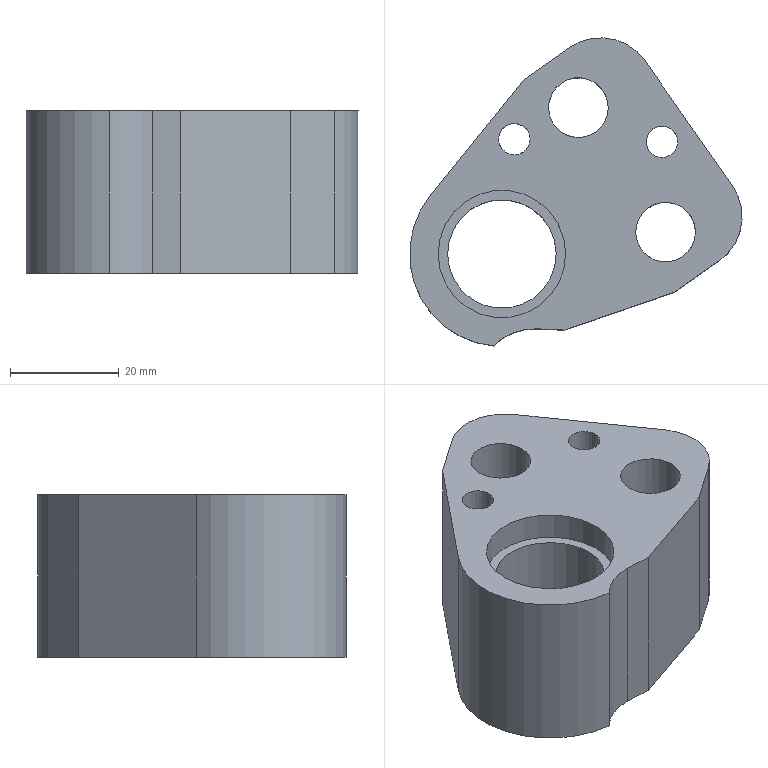Part | NX | features solid 2 | 1 solid | 27 faces | box 61.243 x 56.752 x 30 mm | volume 46658 mm3 | cylinder 14 | plane 13 | commonest cylinder face diameters 20 x3 5.8 x2 8 x2 11 x2 17 x2 21 x1
STEP:
#1=CARTESIAN_POINT('',(-510.031,-151.839,44.));
#2=VERTEX_POINT('',#1);
#3=CARTESIAN_POINT('',(-510.031,-151.839,74.));
#4=VERTEX_POINT('',#3);
#5=CARTESIAN_POINT('',(-510.031,-151.839,44.));
#6=DIRECTION('',(0.,0.,1.));
#7=VECTOR('',#6,1000.);
#8=LINE('',#5,#7);
#9=EDGE_CURVE('',#2,#4,#8,.T.);
#10=ORIENTED_EDGE('',*,*,#9,.F.);
#11=CARTESIAN_POINT('',(-489.755,-144.863,44.));
#12=VERTEX_POINT('',#11);
#13=CARTESIAN_POINT('',(-508.667,-151.37,44.));
#14=DIRECTION('',(-0.9456,-0.3254,0.));
#15=VECTOR('',#14,1000.);
#16=LINE('',#13,#15);
#17=EDGE_CURVE('',#12,#2,#16,.T.);
#18=ORIENTED_EDGE('',*,*,#17,.F.);
#19=CARTESIAN_POINT('',(-489.755,-144.863,74.));
#20=VERTEX_POINT('',#19);
#21=CARTESIAN_POINT('',(-489.755,-144.863,44.));
#22=DIRECTION('',(0.,0.,1.));
#23=VECTOR('',#22,1000.);
#24=LINE('',#21,#23);
#25=EDGE_CURVE('',#12,#20,#24,.T.);
#26=ORIENTED_EDGE('',*,*,#25,.T.);
#27=CARTESIAN_POINT('',(-508.667,-151.37,74.));
#28=DIRECTION('',(0.9456,0.3254,0.));
#29=VECTOR('',#28,1000.);
#30=LINE('',#27,#29);
#31=EDGE_CURVE('',#4,#20,#30,.T.);
#32=ORIENTED_EDGE('',*,*,#31,.F.);
#33=EDGE_LOOP('',(#10,#18,#26,#32));
#34=FACE_BOUND('',#33,.T.);
#35=CARTESIAN_POINT('',(-508.667,-151.37,44.));
#36=DIRECTION('',(-0.3254,0.9456,0.));
#37=DIRECTION('',(0.,0.,-1.));
#38=AXIS2_PLACEMENT_3D('',#35,#36,#37);
#39=PLANE('',#38);
#40=ADVANCED_FACE('',(#34),#39,.F.);
#41=CARTESIAN_POINT('',(-515.152,-151.612,74.));
#42=VERTEX_POINT('',#41);
#43=CARTESIAN_POINT('',(-523.093,-154.751,74.));
#44=VERTEX_POINT('',#43);
#45=CARTESIAN_POINT('',(-515.596,-162.103,74.));
#46=DIRECTION('',(0.,0.,1.));
#47=DIRECTION('',(0.,-1.,0.));
#48=AXIS2_PLACEMENT_3D('',#45,#46,#47);
#49=CIRCLE('',#48,10.5);
#50=EDGE_CURVE('',#42,#44,#49,.T.);
#51=ORIENTED_EDGE('',*,*,#50,.F.);
#52=CARTESIAN_POINT('',(-515.285,-151.606,74.));
#53=DIRECTION('',(0.999,-0.04437,0.));
#54=VECTOR('',#53,1000.);
#55=LINE('',#52,#54);
#56=EDGE_CURVE('',#42,#4,#55,.T.);
#57=ORIENTED_EDGE('',*,*,#56,.T.);
#58=ORIENTED_EDGE('',*,*,#31,.T.);
#59=CARTESIAN_POINT('',(-481.564,-139.127,74.));
#60=VERTEX_POINT('',#59);
#61=CARTESIAN_POINT('',(-500.687,-152.517,74.));
#62=DIRECTION('',(-0.8192,-0.5736,0.));
#63=VECTOR('',#62,1000.);
#64=LINE('',#61,#63);
#65=EDGE_CURVE('',#60,#20,#64,.T.);
#66=ORIENTED_EDGE('',*,*,#65,.F.);
#67=CARTESIAN_POINT('',(-479.108,-125.2,74.));
#68=VERTEX_POINT('',#67);
#69=CARTESIAN_POINT('',(-487.299,-130.936,74.));
#70=DIRECTION('',(0.,0.,1.));
#71=DIRECTION('',(0.,-1.,0.));
#72=AXIS2_PLACEMENT_3D('',#69,#70,#71);
#73=CIRCLE('',#72,10.);
#74=EDGE_CURVE('',#60,#68,#73,.T.);
#75=ORIENTED_EDGE('',*,*,#74,.T.);
#76=CARTESIAN_POINT('',(-495.168,-102.264,74.));
#77=VERTEX_POINT('',#76);
#78=CARTESIAN_POINT('',(-487.138,-113.732,74.));
#79=DIRECTION('',(0.5736,-0.8192,0.));
#80=VECTOR('',#79,1000.);
#81=LINE('',#78,#80);
#82=EDGE_CURVE('',#77,#68,#81,.T.);
#83=ORIENTED_EDGE('',*,*,#82,.F.);
#84=CARTESIAN_POINT('',(-509.095,-99.808,74.));
#85=VERTEX_POINT('',#84);
#86=CARTESIAN_POINT('',(-503.359,-107.999,74.));
#87=DIRECTION('',(0.,0.,1.));
#88=DIRECTION('',(0.,-1.,0.));
#89=AXIS2_PLACEMENT_3D('',#86,#87,#88);
#90=CIRCLE('',#89,10.);
#91=EDGE_CURVE('',#77,#85,#90,.T.);
#92=ORIENTED_EDGE('',*,*,#91,.T.);
#93=CARTESIAN_POINT('',(-517.287,-105.544,74.));
#94=VERTEX_POINT('',#93);
#95=CARTESIAN_POINT('',(-528.218,-113.198,74.));
#96=DIRECTION('',(0.8192,0.5736,0.));
#97=VECTOR('',#96,1000.);
#98=LINE('',#95,#97);
#99=EDGE_CURVE('',#94,#85,#98,.T.);
#100=ORIENTED_EDGE('',*,*,#99,.F.);
#101=CARTESIAN_POINT('',(-534.756,-127.127,74.));
#102=VERTEX_POINT('',#101);
#103=CARTESIAN_POINT('',(-529.87,-121.089,74.));
#104=DIRECTION('',(-0.6291,-0.7773,0.));
#105=VECTOR('',#104,1000.);
#106=LINE('',#103,#105);
#107=EDGE_CURVE('',#94,#102,#106,.T.);
#108=ORIENTED_EDGE('',*,*,#107,.T.);
#109=CARTESIAN_POINT('',(-521.542,-137.822,74.));
#110=DIRECTION('',(0.,0.,-1.));
#111=DIRECTION('',(0.5736,-0.8192,0.));
#112=AXIS2_PLACEMENT_3D('',#109,#110,#111);
#113=CIRCLE('',#112,17.);
#114=EDGE_CURVE('',#44,#102,#113,.T.);
#115=ORIENTED_EDGE('',*,*,#114,.F.);
#116=EDGE_LOOP('',(#51,#57,#58,#66,#75,#83,#92,#100,#108,#115));
#117=FACE_BOUND('',#116,.T.);
#118=CARTESIAN_POINT('',(-490.389,-119.549,74.));
#119=VERTEX_POINT('',#118);
#120=CARTESIAN_POINT('',(-492.053,-117.173,74.));
#121=DIRECTION('',(0.,0.,-1.));
#122=DIRECTION('',(0.5736,-0.8192,0.));
#123=AXIS2_PLACEMENT_3D('',#120,#121,#122);
#124=CIRCLE('',#123,2.9);
#125=EDGE_CURVE('',#119,#119,#124,.T.);
#126=ORIENTED_EDGE('',*,*,#125,.T.);
#127=EDGE_LOOP('',(#126));
#128=FACE_BOUND('',#127,.T.);
#129=CARTESIAN_POINT('',(-517.588,-119.061,74.));
#130=VERTEX_POINT('',#129);
#131=CARTESIAN_POINT('',(-519.251,-116.686,74.));
#132=DIRECTION('',(0.,0.,-1.));
#133=DIRECTION('',(0.5736,-0.8192,0.));
#134=AXIS2_PLACEMENT_3D('',#131,#132,#133);
#135=CIRCLE('',#134,2.9);
#136=EDGE_CURVE('',#130,#130,#135,.T.);
#137=ORIENTED_EDGE('',*,*,#136,.T.);
#138=EDGE_LOOP('',(#137));
#139=FACE_BOUND('',#138,.T.);
#140=CARTESIAN_POINT('',(-504.301,-115.373,74.));
#141=VERTEX_POINT('',#140);
#142=CARTESIAN_POINT('',(-507.455,-110.867,74.));
#143=DIRECTION('',(0.,0.,-1.));
#144=DIRECTION('',(0.5736,-0.8192,0.));
#145=AXIS2_PLACEMENT_3D('',#142,#143,#144);
#146=CIRCLE('',#145,5.5);
#147=EDGE_CURVE('',#141,#141,#146,.T.);
#148=ORIENTED_EDGE('',*,*,#147,.T.);
#149=EDGE_LOOP('',(#148));
#150=FACE_BOUND('',#149,.T.);
#151=CARTESIAN_POINT('',(-488.24,-138.309,74.));
#152=VERTEX_POINT('',#151);
#153=CARTESIAN_POINT('',(-491.395,-133.804,74.));
#154=DIRECTION('',(0.,0.,-1.));
#155=DIRECTION('',(0.5736,-0.8192,0.));
#156=AXIS2_PLACEMENT_3D('',#153,#154,#155);
#157=CIRCLE('',#156,5.5);
#158=EDGE_CURVE('',#152,#152,#157,.T.);
#159=ORIENTED_EDGE('',*,*,#158,.T.);
#160=EDGE_LOOP('',(#159));
#161=FACE_BOUND('',#160,.T.);
#162=CARTESIAN_POINT('',(-514.803,-147.447,74.));
#163=VERTEX_POINT('',#162);
#164=CARTESIAN_POINT('',(-521.542,-137.822,74.));
#165=DIRECTION('',(0.,0.,-1.));
#166=DIRECTION('',(0.5736,-0.8192,0.));
#167=AXIS2_PLACEMENT_3D('',#164,#165,#166);
#168=CIRCLE('',#167,11.75);
#169=EDGE_CURVE('',#163,#163,#168,.T.);
#170=ORIENTED_EDGE('',*,*,#169,.T.);
#171=EDGE_LOOP('',(#170));
#172=FACE_BOUND('',#171,.T.);
#173=CARTESIAN_POINT('',(-514.453,-132.858,74.));
#174=DIRECTION('',(0.,0.,1.));
#175=DIRECTION('',(-0.5736,0.8192,0.));
#176=AXIS2_PLACEMENT_3D('',#173,#174,#175);
#177=PLANE('',#176);
#178=ADVANCED_FACE('',(#117,#128,#139,#150,#161,#172),#177,.T.);
#179=ORIENTED_EDGE('',*,*,#25,.F.);
#180=CARTESIAN_POINT('',(-481.564,-139.127,44.));
#181=VERTEX_POINT('',#180);
#182=CARTESIAN_POINT('',(-500.687,-152.517,44.));
#183=DIRECTION('',(0.8192,0.5736,0.));
#184=VECTOR('',#183,1000.);
#185=LINE('',#182,#184);
#186=EDGE_CURVE('',#12,#181,#185,.T.);
#187=ORIENTED_EDGE('',*,*,#186,.T.);
#188=CARTESIAN_POINT('',(-481.564,-139.127,44.));
#189=DIRECTION('',(0.,0.,1.));
#190=VECTOR('',#189,1000.);
#191=LINE('',#188,#190);
#192=EDGE_CURVE('',#181,#60,#191,.T.);
#193=ORIENTED_EDGE('',*,*,#192,.T.);
#194=ORIENTED_EDGE('',*,*,#65,.T.);
#195=EDGE_LOOP('',(#179,#187,#193,#194));
#196=FACE_BOUND('',#195,.T.);
#197=CARTESIAN_POINT('',(-500.687,-152.517,44.));
#198=DIRECTION('',(0.5736,-0.8192,0.));
#199=DIRECTION('',(0.,0.,1.));
#200=AXIS2_PLACEMENT_3D('',#197,#198,#199);
#201=PLANE('',#200);
#202=ADVANCED_FACE('',(#196),#201,.T.);
#203=CARTESIAN_POINT('',(-523.093,-154.751,44.));
#204=VERTEX_POINT('',#203);
#205=CARTESIAN_POINT('',(-515.152,-151.612,44.));
#206=VERTEX_POINT('',#205);
#207=CARTESIAN_POINT('',(-515.596,-162.103,44.));
#208=DIRECTION('',(0.,0.,-1.));
#209=DIRECTION('',(0.,1.,0.));
#210=AXIS2_PLACEMENT_3D('',#207,#208,#209);
#211=CIRCLE('',#210,10.5);
#212=EDGE_CURVE('',#204,#206,#211,.T.);
#213=ORIENTED_EDGE('',*,*,#212,.F.);
#214=CARTESIAN_POINT('',(-534.756,-127.127,44.));
#215=VERTEX_POINT('',#214);
#216=CARTESIAN_POINT('',(-521.542,-137.822,44.));
#217=DIRECTION('',(0.,0.,1.));
#218=DIRECTION('',(-0.5736,0.8192,0.));
#219=AXIS2_PLACEMENT_3D('',#216,#217,#218);
#220=CIRCLE('',#219,17.);
#221=EDGE_CURVE('',#215,#204,#220,.T.);
#222=ORIENTED_EDGE('',*,*,#221,.F.);
#223=CARTESIAN_POINT('',(-517.287,-105.544,44.));
#224=VERTEX_POINT('',#223);
#225=CARTESIAN_POINT('',(-529.87,-121.089,44.));
#226=DIRECTION('',(0.6291,0.7773,0.));
#227=VECTOR('',#226,1000.);
#228=LINE('',#225,#227);
#229=EDGE_CURVE('',#215,#224,#228,.T.);
#230=ORIENTED_EDGE('',*,*,#229,.T.);
#231=CARTESIAN_POINT('',(-509.095,-99.808,44.));
#232=VERTEX_POINT('',#231);
#233=CARTESIAN_POINT('',(-528.218,-113.198,44.));
#234=DIRECTION('',(-0.8192,-0.5736,0.));
#235=VECTOR('',#234,1000.);
#236=LINE('',#233,#235);
#237=EDGE_CURVE('',#232,#224,#236,.T.);
#238=ORIENTED_EDGE('',*,*,#237,.F.);
#239=CARTESIAN_POINT('',(-495.168,-102.264,44.));
#240=VERTEX_POINT('',#239);
#241=CARTESIAN_POINT('',(-503.359,-107.999,44.));
#242=DIRECTION('',(0.,0.,-1.));
#243=DIRECTION('',(0.,1.,0.));
#244=AXIS2_PLACEMENT_3D('',#241,#242,#243);
#245=CIRCLE('',#244,10.);
#246=EDGE_CURVE('',#232,#240,#245,.T.);
#247=ORIENTED_EDGE('',*,*,#246,.T.);
#248=CARTESIAN_POINT('',(-479.108,-125.2,44.));
#249=VERTEX_POINT('',#248);
#250=CARTESIAN_POINT('',(-487.138,-113.732,44.));
#251=DIRECTION('',(-0.5736,0.8192,0.));
#252=VECTOR('',#251,1000.);
#253=LINE('',#250,#252);
#254=EDGE_CURVE('',#249,#240,#253,.T.);
#255=ORIENTED_EDGE('',*,*,#254,.F.);
#256=CARTESIAN_POINT('',(-487.299,-130.936,44.));
#257=DIRECTION('',(0.,0.,-1.));
#258=DIRECTION('',(0.,1.,0.));
#259=AXIS2_PLACEMENT_3D('',#256,#257,#258);
#260=CIRCLE('',#259,10.);
#261=EDGE_CURVE('',#249,#181,#260,.T.);
#262=ORIENTED_EDGE('',*,*,#261,.T.);
#263=ORIENTED_EDGE('',*,*,#186,.F.);
#264=ORIENTED_EDGE('',*,*,#17,.T.);
#265=CARTESIAN_POINT('',(-515.285,-151.606,44.));
#266=DIRECTION('',(-0.999,0.04437,0.));
#267=VECTOR('',#266,1000.);
#268=LINE('',#265,#267);
#269=EDGE_CURVE('',#2,#206,#268,.T.);
#270=ORIENTED_EDGE('',*,*,#269,.T.);
#271=EDGE_LOOP('',(#213,#222,#230,#238,#247,#255,#262,#263,#264,#270));
#272=FACE_BOUND('',#271,.T.);
#273=CARTESIAN_POINT('',(-494.347,-113.897,44.));
#274=VERTEX_POINT('',#273);
#275=CARTESIAN_POINT('',(-492.053,-117.173,44.));
#276=DIRECTION('',(0.,0.,1.));
#277=DIRECTION('',(-0.5736,0.8192,0.));
#278=AXIS2_PLACEMENT_3D('',#275,#276,#277);
#279=CIRCLE('',#278,4.);
#280=EDGE_CURVE('',#274,#274,#279,.T.);
#281=ORIENTED_EDGE('',*,*,#280,.T.);
#282=EDGE_LOOP('',(#281));
#283=FACE_BOUND('',#282,.T.);
#284=CARTESIAN_POINT('',(-521.546,-113.409,44.));
#285=VERTEX_POINT('',#284);
#286=CARTESIAN_POINT('',(-519.251,-116.686,44.));
#287=DIRECTION('',(0.,0.,1.));
#288=DIRECTION('',(-0.5736,0.8192,0.));
#289=AXIS2_PLACEMENT_3D('',#286,#287,#288);
#290=CIRCLE('',#289,4.);
#291=EDGE_CURVE('',#285,#285,#290,.T.);
#292=ORIENTED_EDGE('',*,*,#291,.T.);
#293=EDGE_LOOP('',(#292));
#294=FACE_BOUND('',#293,.T.);
#295=CARTESIAN_POINT('',(-512.331,-103.905,44.));
#296=VERTEX_POINT('',#295);
#297=CARTESIAN_POINT('',(-507.455,-110.867,44.));
#298=DIRECTION('',(0.,0.,1.));
#299=DIRECTION('',(-0.5736,0.8192,0.));
#300=AXIS2_PLACEMENT_3D('',#297,#298,#299);
#301=CIRCLE('',#300,8.5);
#302=EDGE_CURVE('',#296,#296,#301,.T.);
#303=ORIENTED_EDGE('',*,*,#302,.T.);
#304=EDGE_LOOP('',(#303));
#305=FACE_BOUND('',#304,.T.);
#306=CARTESIAN_POINT('',(-496.271,-126.841,44.));
#307=VERTEX_POINT('',#306);
#308=CARTESIAN_POINT('',(-491.395,-133.804,44.));
#309=DIRECTION('',(0.,0.,1.));
#310=DIRECTION('',(-0.5736,0.8192,0.));
#311=AXIS2_PLACEMENT_3D('',#308,#309,#310);
#312=CIRCLE('',#311,8.5);
#313=EDGE_CURVE('',#307,#307,#312,.T.);
#314=ORIENTED_EDGE('',*,*,#313,.T.);
#315=EDGE_LOOP('',(#314));
#316=FACE_BOUND('',#315,.T.);
#317=CARTESIAN_POINT('',(-527.278,-129.631,44.));
#318=VERTEX_POINT('',#317);
#319=CARTESIAN_POINT('',(-521.542,-137.822,44.));
#320=DIRECTION('',(0.,0.,1.));
#321=DIRECTION('',(-0.5736,0.8192,0.));
#322=AXIS2_PLACEMENT_3D('',#319,#320,#321);
#323=CIRCLE('',#322,10.);
#324=EDGE_CURVE('',#318,#318,#323,.T.);
#325=ORIENTED_EDGE('',*,*,#324,.T.);
#326=EDGE_LOOP('',(#325));
#327=FACE_BOUND('',#326,.T.);
#328=CARTESIAN_POINT('',(-514.453,-132.858,44.));
#329=DIRECTION('',(0.,0.,-1.));
#330=DIRECTION('',(0.5736,-0.8192,0.));
#331=AXIS2_PLACEMENT_3D('',#328,#329,#330);
#332=PLANE('',#331);
#333=ADVANCED_FACE('',(#272,#283,#294,#305,#316,#327),#332,.T.);
#334=CARTESIAN_POINT('',(-517.287,-105.544,44.));
#335=DIRECTION('',(0.,0.,1.));
#336=VECTOR('',#335,1000.);
#337=LINE('',#334,#336);
#338=EDGE_CURVE('',#224,#94,#337,.T.);
#339=ORIENTED_EDGE('',*,*,#338,.T.);
#340=ORIENTED_EDGE('',*,*,#99,.T.);
#341=CARTESIAN_POINT('',(-509.095,-99.808,44.));
#342=DIRECTION('',(0.,0.,1.));
#343=VECTOR('',#342,1000.);
#344=LINE('',#341,#343);
#345=EDGE_CURVE('',#85,#232,#344,.F.);
#346=ORIENTED_EDGE('',*,*,#345,.T.);
#347=ORIENTED_EDGE('',*,*,#237,.T.);
#348=EDGE_LOOP('',(#339,#340,#346,#347));
#349=FACE_BOUND('',#348,.T.);
#350=CARTESIAN_POINT('',(-528.218,-113.198,44.));
#351=DIRECTION('',(-0.5736,0.8192,0.));
#352=DIRECTION('',(0.,0.,-1.));
#353=AXIS2_PLACEMENT_3D('',#350,#351,#352);
#354=PLANE('',#353);
#355=ADVANCED_FACE('',(#349),#354,.T.);
#356=CARTESIAN_POINT('',(-523.093,-154.751,150.));
#357=DIRECTION('',(0.,0.,1.));
#358=VECTOR('',#357,1000.);
#359=LINE('',#356,#358);
#360=EDGE_CURVE('',#44,#204,#359,.F.);
#361=ORIENTED_EDGE('',*,*,#360,.F.);
#362=ORIENTED_EDGE('',*,*,#114,.T.);
#363=CARTESIAN_POINT('',(-534.756,-127.127,74.));
#364=DIRECTION('',(0.,0.,-1.));
#365=VECTOR('',#364,1000.);
#366=LINE('',#363,#365);
#367=EDGE_CURVE('',#102,#215,#366,.T.);
#368=ORIENTED_EDGE('',*,*,#367,.T.);
#369=ORIENTED_EDGE('',*,*,#221,.T.);
#370=EDGE_LOOP('',(#361,#362,#368,#369));
#371=FACE_BOUND('',#370,.T.);
#372=CARTESIAN_POINT('',(-521.542,-137.822,74.));
#373=DIRECTION('',(0.,0.,-1.));
#374=DIRECTION('',(0.5736,-0.8192,0.));
#375=AXIS2_PLACEMENT_3D('',#372,#373,#374);
#376=CYLINDRICAL_SURFACE('',#375,17.);
#377=ADVANCED_FACE('',(#371),#376,.T.);
#378=ORIENTED_EDGE('',*,*,#254,.T.);
#379=CARTESIAN_POINT('',(-495.168,-102.264,44.));
#380=DIRECTION('',(0.,0.,1.));
#381=VECTOR('',#380,1000.);
#382=LINE('',#379,#381);
#383=EDGE_CURVE('',#240,#77,#382,.T.);
#384=ORIENTED_EDGE('',*,*,#383,.T.);
#385=ORIENTED_EDGE('',*,*,#82,.T.);
#386=CARTESIAN_POINT('',(-479.108,-125.2,44.));
#387=DIRECTION('',(0.,0.,1.));
#388=VECTOR('',#387,1000.);
#389=LINE('',#386,#388);
#390=EDGE_CURVE('',#68,#249,#389,.F.);
#391=ORIENTED_EDGE('',*,*,#390,.T.);
#392=EDGE_LOOP('',(#378,#384,#385,#391));
#393=FACE_BOUND('',#392,.T.);
#394=CARTESIAN_POINT('',(-487.138,-113.732,44.));
#395=DIRECTION('',(0.8192,0.5736,0.));
#396=DIRECTION('',(0.,0.,-1.));
#397=AXIS2_PLACEMENT_3D('',#394,#395,#396);
#398=PLANE('',#397);
#399=ADVANCED_FACE('',(#393),#398,.T.);
#400=CARTESIAN_POINT('',(-515.807,-146.014,69.));
#401=VERTEX_POINT('',#400);
#402=CARTESIAN_POINT('',(-521.542,-137.822,69.));
#403=DIRECTION('',(0.,0.,-1.));
#404=DIRECTION('',(0.5736,-0.8192,0.));
#405=AXIS2_PLACEMENT_3D('',#402,#403,#404);
#406=CIRCLE('',#405,10.);
#407=EDGE_CURVE('',#401,#401,#406,.T.);
#408=ORIENTED_EDGE('',*,*,#407,.T.);
#409=EDGE_LOOP('',(#408));
#410=FACE_BOUND('',#409,.T.);
#411=CARTESIAN_POINT('',(-528.282,-128.197,69.));
#412=VERTEX_POINT('',#411);
#413=CARTESIAN_POINT('',(-521.542,-137.822,69.));
#414=DIRECTION('',(0.,0.,1.));
#415=DIRECTION('',(-0.5736,0.8192,0.));
#416=AXIS2_PLACEMENT_3D('',#413,#414,#415);
#417=CIRCLE('',#416,11.75);
#418=EDGE_CURVE('',#412,#412,#417,.T.);
#419=ORIENTED_EDGE('',*,*,#418,.T.);
#420=EDGE_LOOP('',(#419));
#421=FACE_BOUND('',#420,.T.);
#422=CARTESIAN_POINT('',(-521.542,-137.822,69.));
#423=DIRECTION('',(0.,0.,-1.));
#424=DIRECTION('',(0.5736,-0.8192,0.));
#425=AXIS2_PLACEMENT_3D('',#422,#423,#424);
#426=PLANE('',#425);
#427=ADVANCED_FACE('',(#410,#421),#426,.F.);
#428=ORIENTED_EDGE('',*,*,#418,.F.);
#429=EDGE_LOOP('',(#428));
#430=FACE_BOUND('',#429,.T.);
#431=ORIENTED_EDGE('',*,*,#169,.F.);
#432=EDGE_LOOP('',(#431));
#433=FACE_BOUND('',#432,.T.);
#434=CARTESIAN_POINT('',(-521.542,-137.822,74.));
#435=DIRECTION('',(0.,0.,-1.));
#436=DIRECTION('',(0.5736,-0.8192,0.));
#437=AXIS2_PLACEMENT_3D('',#434,#435,#436);
#438=CYLINDRICAL_SURFACE('',#437,11.75);
#439=ADVANCED_FACE('',(#430,#433),#438,.F.);
#440=ORIENTED_EDGE('',*,*,#324,.F.);
#441=EDGE_LOOP('',(#440));
#442=FACE_BOUND('',#441,.T.);
#443=ORIENTED_EDGE('',*,*,#407,.F.);
#444=EDGE_LOOP('',(#443));
#445=FACE_BOUND('',#444,.T.);
#446=CARTESIAN_POINT('',(-521.542,-137.822,69.));
#447=DIRECTION('',(0.,0.,-1.));
#448=DIRECTION('',(0.5736,-0.8192,0.));
#449=AXIS2_PLACEMENT_3D('',#446,#447,#448);
#450=CYLINDRICAL_SURFACE('',#449,10.);
#451=ADVANCED_FACE('',(#442,#445),#450,.F.);
#452=CARTESIAN_POINT('',(-491.395,-139.304,56.));
#453=VERTEX_POINT('',#452);
#454=CARTESIAN_POINT('',(-491.395,-133.804,56.));
#455=DIRECTION('',(0.,0.,1.));
#456=DIRECTION('',(0.,-1.,0.));
#457=AXIS2_PLACEMENT_3D('',#454,#455,#456);
#458=CIRCLE('',#457,5.5);
#459=EDGE_CURVE('',#453,#453,#458,.F.);
#460=ORIENTED_EDGE('',*,*,#459,.T.);
#461=EDGE_LOOP('',(#460));
#462=FACE_BOUND('',#461,.T.);
#463=ORIENTED_EDGE('',*,*,#158,.F.);
#464=EDGE_LOOP('',(#463));
#465=FACE_BOUND('',#464,.T.);
#466=CARTESIAN_POINT('',(-491.395,-133.804,74.));
#467=DIRECTION('',(0.,0.,-1.));
#468=DIRECTION('',(0.5736,-0.8192,0.));
#469=AXIS2_PLACEMENT_3D('',#466,#467,#468);
#470=CYLINDRICAL_SURFACE('',#469,5.5);
#471=ADVANCED_FACE('',(#462,#465),#470,.F.);
#472=CARTESIAN_POINT('',(-486.52,-140.766,56.));
#473=VERTEX_POINT('',#472);
#474=CARTESIAN_POINT('',(-491.395,-133.804,56.));
#475=DIRECTION('',(0.,0.,-1.));
#476=DIRECTION('',(0.5736,-0.8192,0.));
#477=AXIS2_PLACEMENT_3D('',#474,#475,#476);
#478=CIRCLE('',#477,8.5);
#479=EDGE_CURVE('',#473,#473,#478,.T.);
#480=ORIENTED_EDGE('',*,*,#479,.T.);
#481=EDGE_LOOP('',(#480));
#482=FACE_BOUND('',#481,.T.);
#483=ORIENTED_EDGE('',*,*,#459,.F.);
#484=EDGE_LOOP('',(#483));
#485=FACE_BOUND('',#484,.T.);
#486=CARTESIAN_POINT('',(-491.395,-133.804,56.));
#487=DIRECTION('',(0.,0.,1.));
#488=DIRECTION('',(-0.5736,0.8192,0.));
#489=AXIS2_PLACEMENT_3D('',#486,#487,#488);
#490=PLANE('',#489);
#491=ADVANCED_FACE('',(#482,#485),#490,.F.);
#492=ORIENTED_EDGE('',*,*,#313,.F.);
#493=EDGE_LOOP('',(#492));
#494=FACE_BOUND('',#493,.T.);
#495=ORIENTED_EDGE('',*,*,#479,.F.);
#496=EDGE_LOOP('',(#495));
#497=FACE_BOUND('',#496,.T.);
#498=CARTESIAN_POINT('',(-491.395,-133.804,56.));
#499=DIRECTION('',(0.,0.,-1.));
#500=DIRECTION('',(0.5736,-0.8192,0.));
#501=AXIS2_PLACEMENT_3D('',#498,#499,#500);
#502=CYLINDRICAL_SURFACE('',#501,8.5);
#503=ADVANCED_FACE('',(#494,#497),#502,.F.);
#504=CARTESIAN_POINT('',(-507.455,-116.367,56.));
#505=VERTEX_POINT('',#504);
#506=CARTESIAN_POINT('',(-507.455,-110.867,56.));
#507=DIRECTION('',(0.,0.,1.));
#508=DIRECTION('',(0.,-1.,0.));
#509=AXIS2_PLACEMENT_3D('',#506,#507,#508);
#510=CIRCLE('',#509,5.5);
#511=EDGE_CURVE('',#505,#505,#510,.F.);
#512=ORIENTED_EDGE('',*,*,#511,.T.);
#513=EDGE_LOOP('',(#512));
#514=FACE_BOUND('',#513,.T.);
#515=ORIENTED_EDGE('',*,*,#147,.F.);
#516=EDGE_LOOP('',(#515));
#517=FACE_BOUND('',#516,.T.);
#518=CARTESIAN_POINT('',(-507.455,-110.867,74.));
#519=DIRECTION('',(0.,0.,-1.));
#520=DIRECTION('',(0.5736,-0.8192,0.));
#521=AXIS2_PLACEMENT_3D('',#518,#519,#520);
#522=CYLINDRICAL_SURFACE('',#521,5.5);
#523=ADVANCED_FACE('',(#514,#517),#522,.F.);
#524=CARTESIAN_POINT('',(-502.58,-117.83,56.));
#525=VERTEX_POINT('',#524);
#526=CARTESIAN_POINT('',(-507.455,-110.867,56.));
#527=DIRECTION('',(0.,0.,-1.));
#528=DIRECTION('',(0.5736,-0.8192,0.));
#529=AXIS2_PLACEMENT_3D('',#526,#527,#528);
#530=CIRCLE('',#529,8.5);
#531=EDGE_CURVE('',#525,#525,#530,.T.);
#532=ORIENTED_EDGE('',*,*,#531,.T.);
#533=EDGE_LOOP('',(#532));
#534=FACE_BOUND('',#533,.T.);
#535=ORIENTED_EDGE('',*,*,#511,.F.);
#536=EDGE_LOOP('',(#535));
#537=FACE_BOUND('',#536,.T.);
#538=CARTESIAN_POINT('',(-507.455,-110.867,56.));
#539=DIRECTION('',(0.,0.,1.));
#540=DIRECTION('',(-0.5736,0.8192,0.));
#541=AXIS2_PLACEMENT_3D('',#538,#539,#540);
#542=PLANE('',#541);
#543=ADVANCED_FACE('',(#534,#537),#542,.F.);
#544=ORIENTED_EDGE('',*,*,#302,.F.);
#545=EDGE_LOOP('',(#544));
#546=FACE_BOUND('',#545,.T.);
#547=ORIENTED_EDGE('',*,*,#531,.F.);
#548=EDGE_LOOP('',(#547));
#549=FACE_BOUND('',#548,.T.);
#550=CARTESIAN_POINT('',(-507.455,-110.867,56.));
#551=DIRECTION('',(0.,0.,-1.));
#552=DIRECTION('',(0.5736,-0.8192,0.));
#553=AXIS2_PLACEMENT_3D('',#550,#551,#552);
#554=CYLINDRICAL_SURFACE('',#553,8.5);
#555=ADVANCED_FACE('',(#546,#549),#554,.F.);
#556=CARTESIAN_POINT('',(-519.251,-119.586,64.));
#557=VERTEX_POINT('',#556);
#558=CARTESIAN_POINT('',(-519.251,-116.686,64.));
#559=DIRECTION('',(0.,0.,1.));
#560=DIRECTION('',(0.,-1.,0.));
#561=AXIS2_PLACEMENT_3D('',#558,#559,#560);
#562=CIRCLE('',#561,2.9);
#563=EDGE_CURVE('',#557,#557,#562,.F.);
#564=ORIENTED_EDGE('',*,*,#563,.T.);
#565=EDGE_LOOP('',(#564));
#566=FACE_BOUND('',#565,.T.);
#567=ORIENTED_EDGE('',*,*,#136,.F.);
#568=EDGE_LOOP('',(#567));
#569=FACE_BOUND('',#568,.T.);
#570=CARTESIAN_POINT('',(-519.251,-116.686,74.));
#571=DIRECTION('',(0.,0.,-1.));
#572=DIRECTION('',(0.5736,-0.8192,0.));
#573=AXIS2_PLACEMENT_3D('',#570,#571,#572);
#574=CYLINDRICAL_SURFACE('',#573,2.9);
#575=ADVANCED_FACE('',(#566,#569),#574,.F.);
#576=CARTESIAN_POINT('',(-516.957,-119.962,64.));
#577=VERTEX_POINT('',#576);
#578=CARTESIAN_POINT('',(-519.251,-116.686,64.));
#579=DIRECTION('',(0.,0.,-1.));
#580=DIRECTION('',(0.5736,-0.8192,0.));
#581=AXIS2_PLACEMENT_3D('',#578,#579,#580);
#582=CIRCLE('',#581,4.);
#583=EDGE_CURVE('',#577,#577,#582,.T.);
#584=ORIENTED_EDGE('',*,*,#583,.T.);
#585=EDGE_LOOP('',(#584));
#586=FACE_BOUND('',#585,.T.);
#587=ORIENTED_EDGE('',*,*,#563,.F.);
#588=EDGE_LOOP('',(#587));
#589=FACE_BOUND('',#588,.T.);
#590=CARTESIAN_POINT('',(-519.251,-116.686,64.));
#591=DIRECTION('',(0.,0.,1.));
#592=DIRECTION('',(-0.5736,0.8192,0.));
#593=AXIS2_PLACEMENT_3D('',#590,#591,#592);
#594=PLANE('',#593);
#595=ADVANCED_FACE('',(#586,#589),#594,.F.);
#596=ORIENTED_EDGE('',*,*,#291,.F.);
#597=EDGE_LOOP('',(#596));
#598=FACE_BOUND('',#597,.T.);
#599=ORIENTED_EDGE('',*,*,#583,.F.);
#600=EDGE_LOOP('',(#599));
#601=FACE_BOUND('',#600,.T.);
#602=CARTESIAN_POINT('',(-519.251,-116.686,64.));
#603=DIRECTION('',(0.,0.,-1.));
#604=DIRECTION('',(0.5736,-0.8192,0.));
#605=AXIS2_PLACEMENT_3D('',#602,#603,#604);
#606=CYLINDRICAL_SURFACE('',#605,4.);
#607=ADVANCED_FACE('',(#598,#601),#606,.F.);
#608=CARTESIAN_POINT('',(-492.053,-120.073,64.));
#609=VERTEX_POINT('',#608);
#610=CARTESIAN_POINT('',(-492.053,-117.173,64.));
#611=DIRECTION('',(0.,0.,1.));
#612=DIRECTION('',(0.,-1.,0.));
#613=AXIS2_PLACEMENT_3D('',#610,#611,#612);
#614=CIRCLE('',#613,2.9);
#615=EDGE_CURVE('',#609,#609,#614,.F.);
#616=ORIENTED_EDGE('',*,*,#615,.T.);
#617=EDGE_LOOP('',(#616));
#618=FACE_BOUND('',#617,.T.);
#619=ORIENTED_EDGE('',*,*,#125,.F.);
#620=EDGE_LOOP('',(#619));
#621=FACE_BOUND('',#620,.T.);
#622=CARTESIAN_POINT('',(-492.053,-117.173,74.));
#623=DIRECTION('',(0.,0.,-1.));
#624=DIRECTION('',(0.5736,-0.8192,0.));
#625=AXIS2_PLACEMENT_3D('',#622,#623,#624);
#626=CYLINDRICAL_SURFACE('',#625,2.9);
#627=ADVANCED_FACE('',(#618,#621),#626,.F.);
#628=CARTESIAN_POINT('',(-489.759,-120.45,64.));
#629=VERTEX_POINT('',#628);
#630=CARTESIAN_POINT('',(-492.053,-117.173,64.));
#631=DIRECTION('',(0.,0.,-1.));
#632=DIRECTION('',(0.5736,-0.8192,0.));
#633=AXIS2_PLACEMENT_3D('',#630,#631,#632);
#634=CIRCLE('',#633,4.);
#635=EDGE_CURVE('',#629,#629,#634,.T.);
#636=ORIENTED_EDGE('',*,*,#635,.T.);
#637=EDGE_LOOP('',(#636));
#638=FACE_BOUND('',#637,.T.);
#639=ORIENTED_EDGE('',*,*,#615,.F.);
#640=EDGE_LOOP('',(#639));
#641=FACE_BOUND('',#640,.T.);
#642=CARTESIAN_POINT('',(-492.053,-117.173,64.));
#643=DIRECTION('',(0.,0.,1.));
#644=DIRECTION('',(-0.5736,0.8192,0.));
#645=AXIS2_PLACEMENT_3D('',#642,#643,#644);
#646=PLANE('',#645);
#647=ADVANCED_FACE('',(#638,#641),#646,.F.);
#648=ORIENTED_EDGE('',*,*,#280,.F.);
#649=EDGE_LOOP('',(#648));
#650=FACE_BOUND('',#649,.T.);
#651=ORIENTED_EDGE('',*,*,#635,.F.);
#652=EDGE_LOOP('',(#651));
#653=FACE_BOUND('',#652,.T.);
#654=CARTESIAN_POINT('',(-492.053,-117.173,64.));
#655=DIRECTION('',(0.,0.,-1.));
#656=DIRECTION('',(0.5736,-0.8192,0.));
#657=AXIS2_PLACEMENT_3D('',#654,#655,#656);
#658=CYLINDRICAL_SURFACE('',#657,4.);
#659=ADVANCED_FACE('',(#650,#653),#658,.F.);
#660=ORIENTED_EDGE('',*,*,#246,.F.);
#661=ORIENTED_EDGE('',*,*,#345,.F.);
#662=ORIENTED_EDGE('',*,*,#91,.F.);
#663=ORIENTED_EDGE('',*,*,#383,.F.);
#664=EDGE_LOOP('',(#660,#661,#662,#663));
#665=FACE_BOUND('',#664,.T.);
#666=CARTESIAN_POINT('',(-503.359,-107.999,44.));
#667=DIRECTION('',(0.,0.,1.));
#668=DIRECTION('',(0.,-1.,0.));
#669=AXIS2_PLACEMENT_3D('',#666,#667,#668);
#670=CYLINDRICAL_SURFACE('',#669,10.);
#671=ADVANCED_FACE('',(#665),#670,.T.);
#672=ORIENTED_EDGE('',*,*,#261,.F.);
#673=ORIENTED_EDGE('',*,*,#390,.F.);
#674=ORIENTED_EDGE('',*,*,#74,.F.);
#675=ORIENTED_EDGE('',*,*,#192,.F.);
#676=EDGE_LOOP('',(#672,#673,#674,#675));
#677=FACE_BOUND('',#676,.T.);
#678=CARTESIAN_POINT('',(-487.299,-130.936,44.));
#679=DIRECTION('',(0.,0.,1.));
#680=DIRECTION('',(0.,-1.,0.));
#681=AXIS2_PLACEMENT_3D('',#678,#679,#680);
#682=CYLINDRICAL_SURFACE('',#681,10.);
#683=ADVANCED_FACE('',(#677),#682,.T.);
#684=ORIENTED_EDGE('',*,*,#367,.F.);
#685=ORIENTED_EDGE('',*,*,#107,.F.);
#686=ORIENTED_EDGE('',*,*,#338,.F.);
#687=ORIENTED_EDGE('',*,*,#229,.F.);
#688=EDGE_LOOP('',(#684,#685,#686,#687));
#689=FACE_BOUND('',#688,.T.);
#690=CARTESIAN_POINT('',(-529.87,-121.089,44.));
#691=DIRECTION('',(0.7773,-0.6291,0.));
#692=DIRECTION('',(0.,0.,1.));
#693=AXIS2_PLACEMENT_3D('',#690,#691,#692);
#694=PLANE('',#693);
#695=ADVANCED_FACE('',(#689),#694,.F.);
#696=ORIENTED_EDGE('',*,*,#56,.F.);
#697=CARTESIAN_POINT('',(-515.152,-151.612,0.));
#698=DIRECTION('',(0.,0.,1.));
#699=VECTOR('',#698,1000.);
#700=LINE('',#697,#699);
#701=EDGE_CURVE('',#206,#42,#700,.T.);
#702=ORIENTED_EDGE('',*,*,#701,.F.);
#703=ORIENTED_EDGE('',*,*,#269,.F.);
#704=ORIENTED_EDGE('',*,*,#9,.T.);
#705=EDGE_LOOP('',(#696,#702,#703,#704));
#706=FACE_BOUND('',#705,.T.);
#707=CARTESIAN_POINT('',(-515.152,-151.612,0.));
#708=DIRECTION('',(-0.04437,-0.999,0.));
#709=DIRECTION('',(0.999,-0.04437,0.));
#710=AXIS2_PLACEMENT_3D('',#707,#708,#709);
#711=PLANE('',#710);
#712=ADVANCED_FACE('',(#706),#711,.T.);
#713=ORIENTED_EDGE('',*,*,#701,.T.);
#714=ORIENTED_EDGE('',*,*,#50,.T.);
#715=ORIENTED_EDGE('',*,*,#360,.T.);
#716=ORIENTED_EDGE('',*,*,#212,.T.);
#717=EDGE_LOOP('',(#713,#714,#715,#716));
#718=FACE_BOUND('',#717,.T.);
#719=CARTESIAN_POINT('',(-515.596,-162.103,0.));
#720=DIRECTION('',(0.,0.,1.));
#721=DIRECTION('',(1.,0.,0.));
#722=AXIS2_PLACEMENT_3D('',#719,#720,#721);
#723=CYLINDRICAL_SURFACE('',#722,10.5);
#724=ADVANCED_FACE('',(#718),#723,.F.);
#725=CLOSED_SHELL('',(#40,#178,#202,#333,#355,#377,#399,#427,#439,#451,#471,#491,#503,#523,#543,#555,#575,#595,#607,#627,#647,#659,#671,#683,#695,#712,#724));
#726=MANIFOLD_SOLID_BREP('',#725);
#727=(LENGTH_UNIT()NAMED_UNIT(*)SI_UNIT(.MILLI.,.METRE.));
#728=UNCERTAINTY_MEASURE_WITH_UNIT(LENGTH_MEASURE(0.00001),#727,'','');
#729=(NAMED_UNIT(*)PLANE_ANGLE_UNIT()SI_UNIT($,.RADIAN.));
#730=(NAMED_UNIT(*)SI_UNIT($,.STERADIAN.)SOLID_ANGLE_UNIT());
#731=(GEOMETRIC_REPRESENTATION_CONTEXT(3)GLOBAL_UNCERTAINTY_ASSIGNED_CONTEXT((#728))GLOBAL_UNIT_ASSIGNED_CONTEXT((#727,#729,#730))REPRESENTATION_CONTEXT('',''));
#732=ADVANCED_BREP_SHAPE_REPRESENTATION('',(#726),#731);